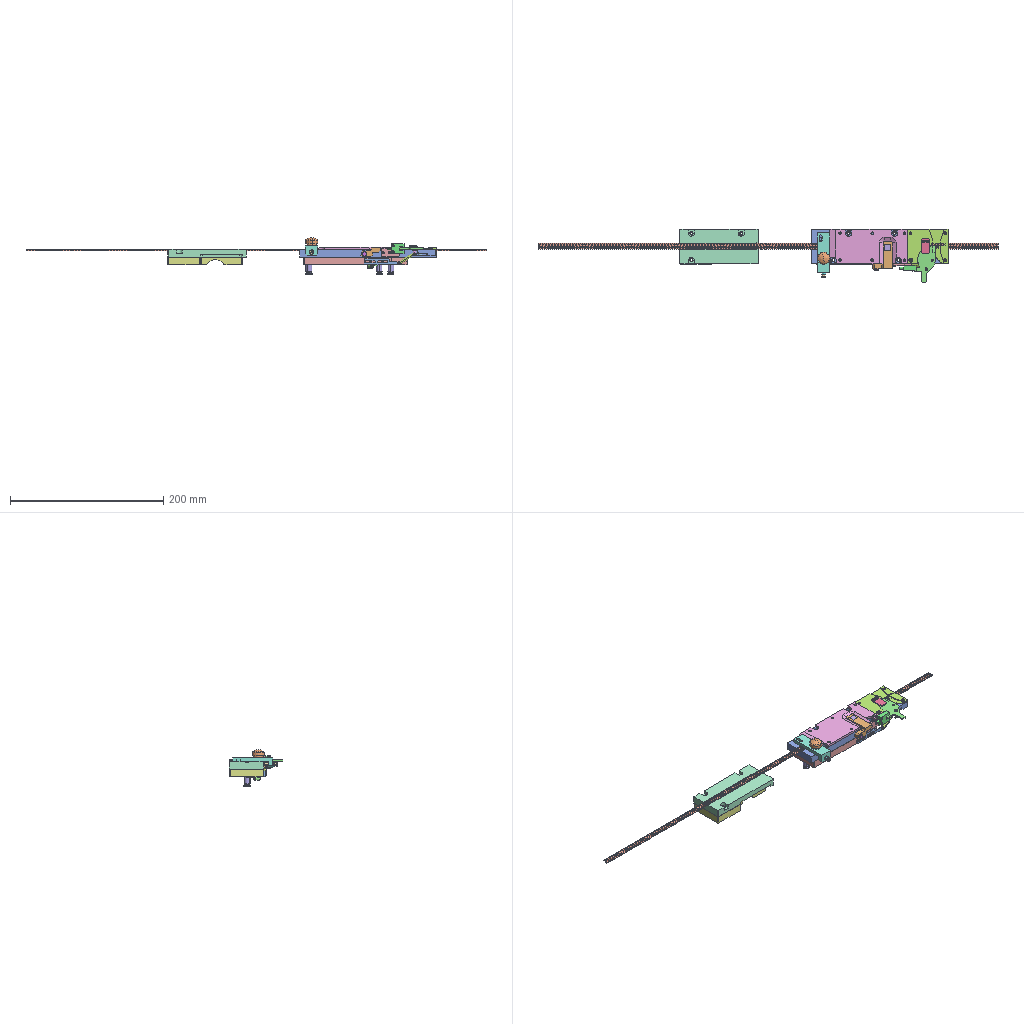Assembly | SolidWorks | 29 different items | 35 placed | box 600 x 69 x 48 mm
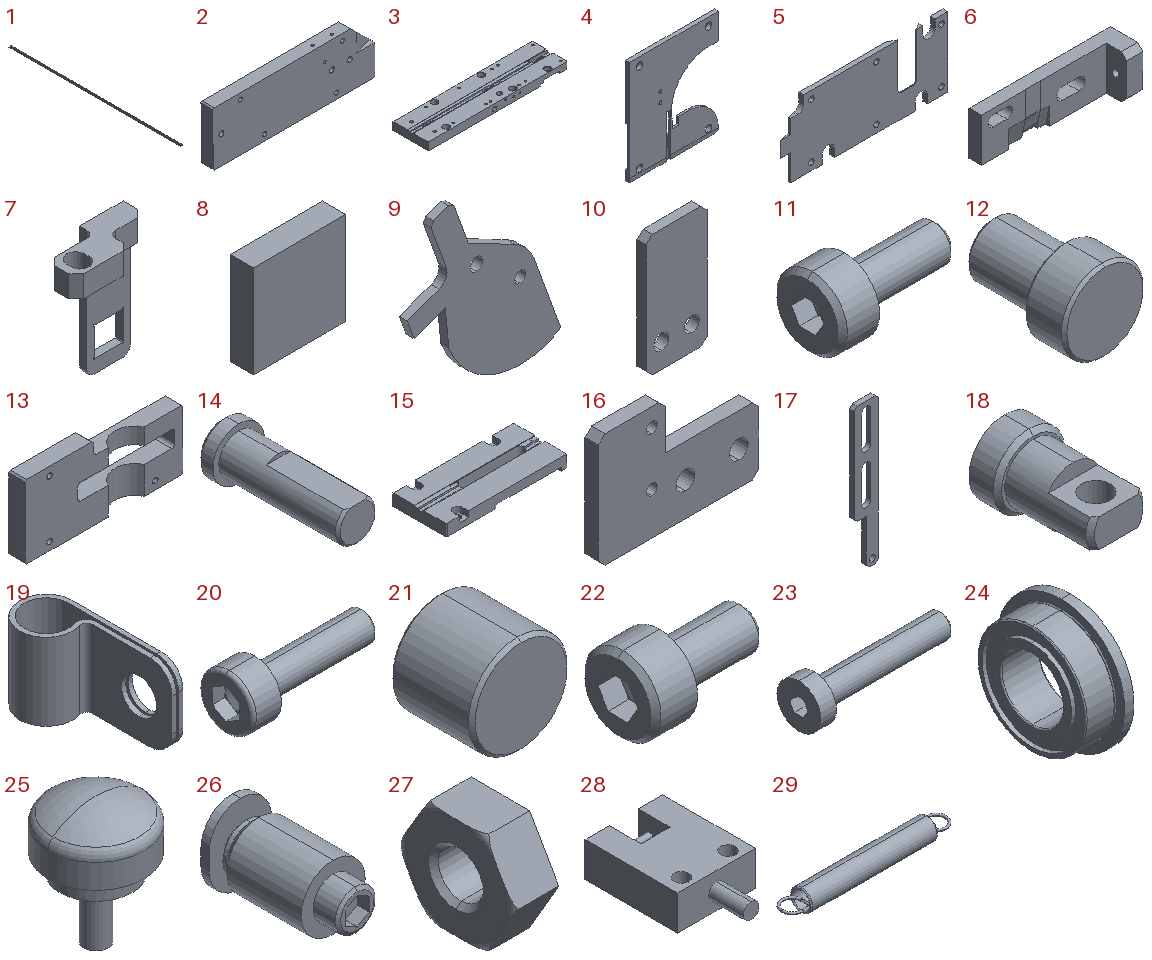Parts list (item | quantity | size | volume | features):
1 | x1 | 8 x 600 x 1.5 mm | 1218 mm3 | features ICE 4, LPattern 4, Extrusion 1
2 | x1 | 135 x 10 x 45 mm | 55764 mm3 | features ICE 14, HoleWzd 6, Chamfer 3, 3DProfileFeature 2, Extrusion 1, Fillet 1, LPattern 1
3 | x1 | 178 x 45 x 10 mm | 72367 mm3 | features ICE 30, HoleWzd 8, Chamfer 7, Fillet 6, 3DProfileFeature 4, Cut 4, Extrusion 1
4 | x1 | 45 x 2 x 53 mm | 3126 mm3 | features ICE 8, Chamfer 4, Extrusion 1, Fillet 1, HoleWzd 1
5 | x1 | 108 x 3 x 45 mm | 11001 mm3 | features ICE 6, Chamfer 1, Cut 1, Extrusion 1, Fillet 1
6 | x1 | 52 x 12 x 16 mm | 3986 mm3 | features ICE 6, Chamfer 2, Fillet 2, 3DProfileFeature 1, Extrusion 1, HoleWzd 1
7 | x1 | 25 x 12 x 35.5 mm | 1512 mm3 | features ICE 7, Fillet 2, 3DProfileFeature 1, Chamfer 1, Extrusion 1, HoleWzd 1
8 | x1 | 8 x 2 x 8 mm | 128 mm3 | features Extrusion 1
9 | x1 | 38.392 x 2 x 43.344 mm | 1473 mm3 | features ICE 14, Fillet 4, Chamfer 3, Extrusion 1
10 | x1 | 10 x 1.5 x 20 mm | 282.274 mm3 | features 3DProfileFeature 1, Chamfer 1, Extrusion 1, HoleWzd 1
11 | x2 | 7 x 3.8 x 3.8 mm | 35.783 mm3 | features ICE 1, RevCut 1, Revolution 1
12 | x1 | 6 x 8.2 x 6 mm | 132.025 mm3 | features Chamfer 2, Extrusion 1, HoleWzd 1, ICE 1
13 | x1 | 97 x 10 x 45 mm | 29685 mm3 | features ICE 9, 3DProfileFeature 2, Fillet 2, HoleWzd 2, Chamfer 1, Extrusion 1
14 | x1 | 6.5 x 17 x 6.5 mm | 347.697 mm3 | features Chamfer 2, ICE 2, Extrusion 1
15 | x1 | 102 x 45 x 10 mm | 38830 mm3 | features ICE 27, Fillet 10, Chamfer 8, HoleWzd 8, 3DProfileFeature 4, Cut 4, Extrusion 1
16 | x1 | 24 x 2 x 17 mm | 582.327 mm3 | features ICE 2, Chamfer 1, Extrusion 1, HoleWzd 1
17 | x1 | 8 x 1.5 x 48 mm | 366.332 mm3 | features ICE 3, Chamfer 1, Extrusion 1, HoleWzd 1
18 | x1 | 5 x 8 x 5 mm | 68.475 mm3 | features ICE 3, Chamfer 1, Extrusion 1, HoleWzd 1
19 | x1 | 4.8 x 12.4 x 7 mm | 75.143 mm3 | features Extrusion 1, Fillet 1, ICE 1
20 | x3 | 7.6 x 3 x 3 mm | 21.652 mm3 | features Fillet 2, RevCut 2, Boss 1, Chamfer 1, Cut 1, Extrusion 1, LPattern 1
21 | x1 | 6 x 5 x 6 mm | 140.634 mm3 | features Chamfer 1, Extrusion 1
22 | x1 | 9 x 5.5 x 5.5 mm | 103.495 mm3 | features ICE 1, RevCut 1, Revolution 1
23 | x1 | 18 x 5.5 x 5.5 mm | 154.645 mm3 | features ICE 1, RevCut 1, Revolution 1
24 | x2 | 2.5 x 8.2 x 8.2 mm | 67.212 mm3 | features RefAxis 3, 3DProfileFeature 1, Revolution 1
25 | x1 | 16 x 16 x 21 mm | 1779 mm3 | features ICE 2, Dome 1, Extrusion 1, Fillet 1
26 | x3 | 8 x 15.6 x 9.8 mm | 520.13 mm3 | features BaseBody 1
27 | x1 | 2.4 x 6.351 x 5.5 mm | 50.814 mm3 | features RefAxis 3, 3DProfileFeature 1, ICE 1, RevCut 1, Revolution 1
28 | x1 | 13.4 x 22 x 6 mm | 1101 mm3 | features ICE 3, Extrusion 1, HoleWzd 1
29 | x1 | 30.8 x 4 x 4 mm | 108.92 mm3 | features Revolution 5, RefAxis 1
Mates (type | each side: item.copy, entity, surface, feature):
Coincident | 3.1 face plane Boss-Extrude1 | 2.1 face plane Boss-Extrude1
Coincident | 3.1 face plane Cut-Extrude2 | 1.1 face plane Boss-Extrude1
DistanceDim | 1.1 face plane Boss-Extrude1 | 3.1 face plane Cut-Extrude2
Coincident | 2.1 face plane Boss-Extrude1 | 3.1 face plane Boss-Extrude1
DistanceDim | 3.1 face plane Boss-Extrude1 | 1.1 face plane LPattern2
Coincident | 3.1 face plane Boss-Extrude1 | 4.1 face plane Boss-Extrude1 | 3 times
Coincident | 3.1 face plane Boss-Extrude1 | 5.1 face plane Boss-Extrude1 | 2 times
Coincident | 3.1 face plane Boss-Extrude1 | 6.1 face plane Boss-Extrude1
Coincident | 5.1 face plane Boss-Extrude1 | 6.1 face plane Boss-Extrude1
DistanceDim | 6.1 face plane Boss-Extrude1 | 3.1 face plane Boss-Extrude1
Coincident | 7.1 face plane Boss-Extrude1 | 8.1 face plane Boss-Extrude1
Coincident | 7.1 face plane Cut-Extrude2 | 8.1 face plane Boss-Extrude1 | 2 times
Coincident | 3.1 face plane Boss-Extrude1 | 9.1 face plane Boss-Extrude1
Concentric | 4.1 face cylinder Cut-Extrude4 | 9.1 face cylinder Boss-Extrude1
Coincident | 9.1 face plane Boss-Extrude1 | 10.1 face plane Boss-Extrude1
Coincident | 10.1 face plane Boss-Extrude1 | 11.1 face plane Revolve1
Concentric | 10.1 face cylinder Ø2.5 (2.5) Diameter Hole1 | 11.1 face cylinder Revolve1
Coincident | 10.1 face plane Boss-Extrude1 | 11.2 face plane Revolve1
Concentric | 10.1 face cylinder Ø2.5 (2.5) Diameter Hole1 | 11.2 face cylinder Revolve1
Coincident | 4.1 face plane Boss-Extrude1 | 22.1 face plane Revolve1
Concentric | 4.1 face cylinder Cut-Extrude6 | 22.1 face cylinder Revolve1
DistanceDim | 10.1 face plane Boss-Extrude1 | 3.1 face plane Boss-Extrude1 | 2 times
Concentric | 3.1 face cylinder Cut-Extrude12 | 12.1 face cylinder Boss-Extrude1
Coincident | 6.1 face plane Boss-Extrude2 | 27.1 face plane Revolve1
Concentric | 6.1 face cylinder M3 Tapped Hole1 | 27.1 face cylinder Cut-Revolve1
Concentric | 27.1 face cylinder Cut-Revolve1 | 23.1 face cylinder Revolve1
DistanceDim | 23.1 face plane Revolve1 | 27.1 face plane Revolve1
Coincident | 3.1 face plane Boss-Extrude1 | 13.1 face plane Boss-Extrude1 | 2 times
Concentric | 2.1 face cylinder M4 Tapped Hole1 | 3.1 face cylinder Cut-Extrude21
Coincident | 4.1 face plane Boss-Extrude2 | 5.1 face plane Cut-Extrude2
Coincident | 7.1 face plane Cut-Extrude4 | 14.1 face plane Boss-Extrude2
Coincident | 3.1 face plane Boss-Extrude1 | 7.1 face plane Boss-Extrude2
Coincident | 3.1 face plane Hole size per hex bolt grade C type 1 | 21.1 face plane Boss-Extrude1
Concentric | 3.1 face cylinder Hole size per hex bolt grade C type 1 | 21.1 face cylinder Boss-Extrude1
Parallel | 4.1 face plane Boss-Extrude1 | 9.1 face plane Cut-Extrude1
Concentric | 13.1 face cylinder M4 Tapped Hole1 | 15.1 face cylinder Cut-Extrude24 | 2 times
Coincident | 13.1 face plane Boss-Extrude1 | 15.1 face plane Boss-Extrude1
DistanceDim | 28.1 face plane Boss-Extrude1 | 3.1 face plane Boss-Extrude1 | 3 times
Coincident | 2.1 face plane Boss-Extrude1 | 16.1 face plane Boss-Extrude1
Coincident | 28.1 face plane Boss-Extrude1 | 16.1 face plane Boss-Extrude1 | 2 times
Coincident | 2.1 face plane Boss-Extrude1 | 17.1 face plane Boss-Extrude1 | 2 times
Concentric | 3.1 face cylinder Cut-Extrude35 | 14.1 face cylinder Boss-Extrude1
Coincident | 3.1 face plane Boss-Extrude1 | 24.1 face plane Revolve1
DistanceDim | 3.1 face plane Cut-Extrude15 | 24.2 face plane Revolve1
Concentric | 3.1 face cylinder Cut-Extrude12 | 24.2 face cylinder Revolve1
Coincident | 12.1 face plane Boss-Extrude1 | 24.1 face plane Revolve1
DistanceDim | 17.1 face plane Boss-Extrude1 | 2.1 face plane Boss-Extrude1
Coincident | 9.1 face plane Boss-Extrude1 | 18.1 face plane Boss-Extrude2
Coincident | 17.1 face plane Boss-Extrude1 | 29.1 plane
Concentric | 9.1 face cylinder Cut-Extrude10 | 18.1 face cylinder M3 Tapped Hole1
Concentric | 9.1 face cylinder Cut-Extrude10 | 20.1 face cylinder BaseBody
Coincident | 9.1 face plane Boss-Extrude1 | 20.1 face plane BaseHead
Tangent | 7.1 face plane Cut-Extrude8 | 14.1 face cylinder Boss-Extrude1
Concentric | 3.1 face cylinder M4 Tapped Hole2 | 25.1 face cylinder Boss-Extrude1
DistanceDim | 25.1 face plane Boss-Extrude2 | 6.1 face plane Boss-Extrude1
Coincident | 2.1 face plane Boss-Extrude1 | 26.1 face plane Input 1
Coincident | 2.1 face plane Boss-Extrude1 | 26.2 face plane Input 1
Coincident | 2.1 face plane Boss-Extrude1 | 26.3 face plane Input 1
Concentric | 2.1 face cylinder M5 Tapped Hole3 | 26.3 face cylinder Input 1
DistanceDim | 15.1 face plane Cut-Extrude34 | 3.1 face plane Cut-Extrude34
Concentric | 2.1 face cylinder M2.5 Tapped Hole1 | 20.2 face cylinder BaseBody
Concentric | 2.1 face cylinder M2.5 Tapped Hole1 | 20.3 face cylinder BaseBody
Coincident | 17.1 face plane Boss-Extrude1 | 20.2 face plane BaseHead
Coincident | 17.1 face plane Boss-Extrude1 | 20.3 face plane BaseHead
Coincident | 2.1 face plane Boss-Extrude1 | 19.1 face plane Boss-Extrude1
Concentric | 2.1 face cylinder M3 Tapped Hole1 | 19.1 face cylinder Cut-Extrude1
Concentric | 2.1 face cylinder M5 Tapped Hole4 | 26.1 face cylinder Input 1